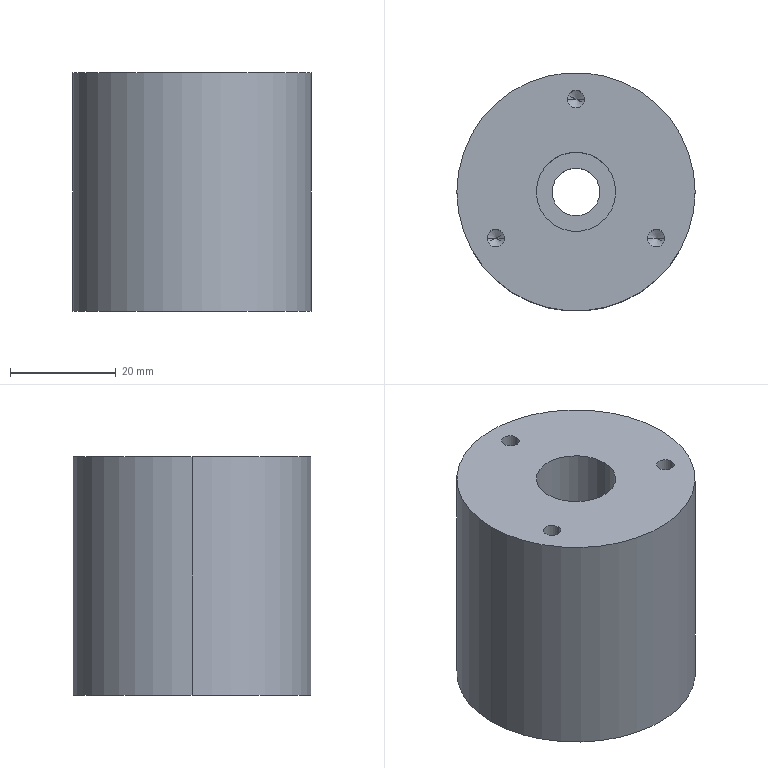Part | STEP file | Caster seat | 1 solid | 21 faces | box 45 x 45 x 45 mm | volume 66141 mm3 | cylinder 12 | cone 6 | plane 3 | commonest cylinder face diameters 3.3 x6 9 x2 15 x2 45 x2
STEP:
#1=CARTESIAN_POINT('',(0.,0.,0.));
#2=DIRECTION('',(0.,0.,1.));
#3=DIRECTION('',(1.,0.,0.));
#4=AXIS2_PLACEMENT_3D('',#1,#2,#3);
#5=CARTESIAN_POINT('',(7.5,0.,25.));
#6=VERTEX_POINT('',#5);
#7=CARTESIAN_POINT('',(7.5,0.,45.));
#8=VERTEX_POINT('',#7);
#9=CARTESIAN_POINT('',(7.5,0.,45.));
#10=DIRECTION('',(0.,0.,1.));
#11=VECTOR('',#10,1.);
#12=LINE('',#9,#11);
#13=CARTESIAN_POINT('',(0.,0.,45.));
#14=DIRECTION('',(0.,0.,1.));
#15=DIRECTION('',(1.,0.,0.));
#16=AXIS2_PLACEMENT_3D('',#13,#14,#15);
#17=CYLINDRICAL_SURFACE('',#16,7.5);
#18=CARTESIAN_POINT('',(6.283,0.));
#19=DIRECTION('',(0.,1.));
#20=VECTOR('',#19,1.);
#21=LINE('',#18,#20);
#22=(GEOMETRIC_REPRESENTATION_CONTEXT(2)PARAMETRIC_REPRESENTATION_CONTEXT()REPRESENTATION_CONTEXT('',''));
#23=DEFINITIONAL_REPRESENTATION('',(#21),#22);
#24=PCURVE('',#17,#23);
#25=CARTESIAN_POINT('',(0.,0.,45.));
#26=DIRECTION('',(0.,0.,1.));
#27=DIRECTION('',(1.,0.,0.));
#28=AXIS2_PLACEMENT_3D('',#25,#26,#27);
#29=CYLINDRICAL_SURFACE('',#28,7.5);
#30=CARTESIAN_POINT('',(0.,0.));
#31=DIRECTION('',(0.,1.));
#32=VECTOR('',#31,1.);
#33=LINE('',#30,#32);
#34=(GEOMETRIC_REPRESENTATION_CONTEXT(2)PARAMETRIC_REPRESENTATION_CONTEXT()REPRESENTATION_CONTEXT('',''));
#35=DEFINITIONAL_REPRESENTATION('',(#33),#34);
#36=PCURVE('',#29,#35);
#37=SURFACE_CURVE('',#12,(#24,#36),.PCURVE_S1.);
#38=EDGE_CURVE('',#6,#8,#37,.T.);
#39=ORIENTED_EDGE('',*,*,#38,.T.);
#40=CARTESIAN_POINT('',(-7.5,0.,45.));
#41=VERTEX_POINT('',#40);
#42=CARTESIAN_POINT('',(0.,0.,45.));
#43=DIRECTION('',(0.,0.,1.));
#44=DIRECTION('',(1.,0.,0.));
#45=AXIS2_PLACEMENT_3D('',#42,#43,#44);
#46=CIRCLE('',#45,7.5);
#47=CARTESIAN_POINT('',(0.,0.));
#48=DIRECTION('',(1.,0.));
#49=VECTOR('',#48,1.);
#50=LINE('',#47,#49);
#51=(GEOMETRIC_REPRESENTATION_CONTEXT(2)PARAMETRIC_REPRESENTATION_CONTEXT()REPRESENTATION_CONTEXT('',''));
#52=DEFINITIONAL_REPRESENTATION('',(#50),#51);
#53=PCURVE('',#17,#52);
#54=CARTESIAN_POINT('',(0.,0.,45.));
#55=DIRECTION('',(0.,0.,1.));
#56=DIRECTION('',(1.,0.,0.));
#57=AXIS2_PLACEMENT_3D('',#54,#55,#56);
#58=PLANE('',#57);
#59=CARTESIAN_POINT('',(0.,0.));
#60=DIRECTION('',(1.,0.));
#61=AXIS2_PLACEMENT_2D('',#59,#60);
#62=CIRCLE('',#61,7.5);
#63=(GEOMETRIC_REPRESENTATION_CONTEXT(2)PARAMETRIC_REPRESENTATION_CONTEXT()REPRESENTATION_CONTEXT('',''));
#64=DEFINITIONAL_REPRESENTATION('',(#62),#63);
#65=PCURVE('',#58,#64);
#66=SURFACE_CURVE('',#46,(#53,#65),.PCURVE_S1.);
#67=EDGE_CURVE('',#41,#8,#66,.T.);
#68=ORIENTED_EDGE('',*,*,#67,.F.);
#69=CARTESIAN_POINT('',(-7.5,0.,25.));
#70=VERTEX_POINT('',#69);
#71=CARTESIAN_POINT('',(-7.5,0.,45.));
#72=DIRECTION('',(0.,0.,1.));
#73=VECTOR('',#72,1.);
#74=LINE('',#71,#73);
#75=CARTESIAN_POINT('',(3.142,0.));
#76=DIRECTION('',(0.,1.));
#77=VECTOR('',#76,1.);
#78=LINE('',#75,#77);
#79=(GEOMETRIC_REPRESENTATION_CONTEXT(2)PARAMETRIC_REPRESENTATION_CONTEXT()REPRESENTATION_CONTEXT('',''));
#80=DEFINITIONAL_REPRESENTATION('',(#78),#79);
#81=PCURVE('',#17,#80);
#82=CARTESIAN_POINT('',(3.142,0.));
#83=DIRECTION('',(0.,1.));
#84=VECTOR('',#83,1.);
#85=LINE('',#82,#84);
#86=(GEOMETRIC_REPRESENTATION_CONTEXT(2)PARAMETRIC_REPRESENTATION_CONTEXT()REPRESENTATION_CONTEXT('',''));
#87=DEFINITIONAL_REPRESENTATION('',(#85),#86);
#88=PCURVE('',#29,#87);
#89=SURFACE_CURVE('',#74,(#81,#88),.PCURVE_S1.);
#90=EDGE_CURVE('',#70,#41,#89,.T.);
#91=ORIENTED_EDGE('',*,*,#90,.F.);
#92=CARTESIAN_POINT('',(0.,0.,25.));
#93=DIRECTION('',(0.,0.,1.));
#94=DIRECTION('',(1.,0.,0.));
#95=AXIS2_PLACEMENT_3D('',#92,#93,#94);
#96=CIRCLE('',#95,7.5);
#97=CARTESIAN_POINT('',(0.,-20.));
#98=DIRECTION('',(1.,0.));
#99=VECTOR('',#98,1.);
#100=LINE('',#97,#99);
#101=(GEOMETRIC_REPRESENTATION_CONTEXT(2)PARAMETRIC_REPRESENTATION_CONTEXT()REPRESENTATION_CONTEXT('',''));
#102=DEFINITIONAL_REPRESENTATION('',(#100),#101);
#103=PCURVE('',#17,#102);
#104=CARTESIAN_POINT('',(4.5,0.,25.));
#105=DIRECTION('',(0.,0.,-1.));
#106=DIRECTION('',(-1.,0.,0.));
#107=AXIS2_PLACEMENT_3D('',#104,#105,#106);
#108=PLANE('',#107);
#109=CARTESIAN_POINT('',(-3.,0.));
#110=CARTESIAN_POINT('',(-3.,12.99));
#111=CARTESIAN_POINT('',(8.25,6.495));
#112=CARTESIAN_POINT('',(19.5,0.));
#113=CARTESIAN_POINT('',(8.25,-6.495));
#114=CARTESIAN_POINT('',(-3.,-12.99));
#115=CARTESIAN_POINT('',(-3.,0.));
#116=(BOUNDED_CURVE()B_SPLINE_CURVE(2,(#109,#110,#111,#112,#113,#114,#115),.UNSPECIFIED.,.T.,.F.)B_SPLINE_CURVE_WITH_KNOTS((1,2,2,2,2,1),(-2.094,0.,2.094,4.189,6.283,8.378),.UNSPECIFIED.)CURVE()GEOMETRIC_REPRESENTATION_ITEM()RATIONAL_B_SPLINE_CURVE((1.,0.5,1.,0.5,1.,0.5,1.))REPRESENTATION_ITEM(''));
#117=(GEOMETRIC_REPRESENTATION_CONTEXT(2)PARAMETRIC_REPRESENTATION_CONTEXT()REPRESENTATION_CONTEXT('',''));
#118=DEFINITIONAL_REPRESENTATION('',(#116),#117);
#119=PCURVE('',#108,#118);
#120=SURFACE_CURVE('',#96,(#103,#119),.PCURVE_S1.);
#121=EDGE_CURVE('',#70,#6,#120,.T.);
#122=ORIENTED_EDGE('',*,*,#121,.T.);
#123=EDGE_LOOP('',(#39,#68,#91,#122));
#124=FACE_BOUND('',#123,.F.);
#125=ADVANCED_FACE('',(#124),#17,.F.);
#126=CARTESIAN_POINT('',(4.5,0.,0.));
#127=VERTEX_POINT('',#126);
#128=CARTESIAN_POINT('',(4.5,0.,25.));
#129=VERTEX_POINT('',#128);
#130=CARTESIAN_POINT('',(4.5,0.,45.));
#131=DIRECTION('',(0.,0.,1.));
#132=VECTOR('',#131,1.);
#133=LINE('',#130,#132);
#134=CARTESIAN_POINT('',(0.,0.,45.));
#135=DIRECTION('',(0.,0.,1.));
#136=DIRECTION('',(1.,0.,0.));
#137=AXIS2_PLACEMENT_3D('',#134,#135,#136);
#138=CYLINDRICAL_SURFACE('',#137,4.5);
#139=CARTESIAN_POINT('',(6.283,0.));
#140=DIRECTION('',(0.,1.));
#141=VECTOR('',#140,1.);
#142=LINE('',#139,#141);
#143=(GEOMETRIC_REPRESENTATION_CONTEXT(2)PARAMETRIC_REPRESENTATION_CONTEXT()REPRESENTATION_CONTEXT('',''));
#144=DEFINITIONAL_REPRESENTATION('',(#142),#143);
#145=PCURVE('',#138,#144);
#146=CARTESIAN_POINT('',(0.,0.,45.));
#147=DIRECTION('',(0.,0.,1.));
#148=DIRECTION('',(1.,0.,0.));
#149=AXIS2_PLACEMENT_3D('',#146,#147,#148);
#150=CYLINDRICAL_SURFACE('',#149,4.5);
#151=CARTESIAN_POINT('',(0.,0.));
#152=DIRECTION('',(0.,1.));
#153=VECTOR('',#152,1.);
#154=LINE('',#151,#153);
#155=(GEOMETRIC_REPRESENTATION_CONTEXT(2)PARAMETRIC_REPRESENTATION_CONTEXT()REPRESENTATION_CONTEXT('',''));
#156=DEFINITIONAL_REPRESENTATION('',(#154),#155);
#157=PCURVE('',#150,#156);
#158=SURFACE_CURVE('',#133,(#145,#157),.PCURVE_S1.);
#159=EDGE_CURVE('',#127,#129,#158,.T.);
#160=ORIENTED_EDGE('',*,*,#159,.T.);
#161=CARTESIAN_POINT('',(-4.5,0.,25.));
#162=VERTEX_POINT('',#161);
#163=CARTESIAN_POINT('',(0.,0.,25.));
#164=DIRECTION('',(0.,0.,1.));
#165=DIRECTION('',(1.,0.,0.));
#166=AXIS2_PLACEMENT_3D('',#163,#164,#165);
#167=CIRCLE('',#166,4.5);
#168=CARTESIAN_POINT('',(0.,-20.));
#169=DIRECTION('',(1.,0.));
#170=VECTOR('',#169,1.);
#171=LINE('',#168,#170);
#172=(GEOMETRIC_REPRESENTATION_CONTEXT(2)PARAMETRIC_REPRESENTATION_CONTEXT()REPRESENTATION_CONTEXT('',''));
#173=DEFINITIONAL_REPRESENTATION('',(#171),#172);
#174=PCURVE('',#138,#173);
#175=CARTESIAN_POINT('',(0.,0.));
#176=CARTESIAN_POINT('',(0.,7.794));
#177=CARTESIAN_POINT('',(6.75,3.897));
#178=CARTESIAN_POINT('',(13.5,0.));
#179=CARTESIAN_POINT('',(6.75,-3.897));
#180=CARTESIAN_POINT('',(0.,-7.794));
#181=CARTESIAN_POINT('',(0.,0.));
#182=(BOUNDED_CURVE()B_SPLINE_CURVE(2,(#175,#176,#177,#178,#179,#180,#181),.UNSPECIFIED.,.T.,.F.)B_SPLINE_CURVE_WITH_KNOTS((1,2,2,2,2,1),(-2.094,0.,2.094,4.189,6.283,8.378),.UNSPECIFIED.)CURVE()GEOMETRIC_REPRESENTATION_ITEM()RATIONAL_B_SPLINE_CURVE((1.,0.5,1.,0.5,1.,0.5,1.))REPRESENTATION_ITEM(''));
#183=(GEOMETRIC_REPRESENTATION_CONTEXT(2)PARAMETRIC_REPRESENTATION_CONTEXT()REPRESENTATION_CONTEXT('',''));
#184=DEFINITIONAL_REPRESENTATION('',(#182),#183);
#185=PCURVE('',#108,#184);
#186=SURFACE_CURVE('',#167,(#174,#185),.PCURVE_S1.);
#187=EDGE_CURVE('',#162,#129,#186,.T.);
#188=ORIENTED_EDGE('',*,*,#187,.F.);
#189=CARTESIAN_POINT('',(-4.5,0.,0.));
#190=VERTEX_POINT('',#189);
#191=CARTESIAN_POINT('',(-4.5,0.,45.));
#192=DIRECTION('',(0.,0.,1.));
#193=VECTOR('',#192,1.);
#194=LINE('',#191,#193);
#195=CARTESIAN_POINT('',(3.142,0.));
#196=DIRECTION('',(0.,1.));
#197=VECTOR('',#196,1.);
#198=LINE('',#195,#197);
#199=(GEOMETRIC_REPRESENTATION_CONTEXT(2)PARAMETRIC_REPRESENTATION_CONTEXT()REPRESENTATION_CONTEXT('',''));
#200=DEFINITIONAL_REPRESENTATION('',(#198),#199);
#201=PCURVE('',#138,#200);
#202=CARTESIAN_POINT('',(3.142,0.));
#203=DIRECTION('',(0.,1.));
#204=VECTOR('',#203,1.);
#205=LINE('',#202,#204);
#206=(GEOMETRIC_REPRESENTATION_CONTEXT(2)PARAMETRIC_REPRESENTATION_CONTEXT()REPRESENTATION_CONTEXT('',''));
#207=DEFINITIONAL_REPRESENTATION('',(#205),#206);
#208=PCURVE('',#150,#207);
#209=SURFACE_CURVE('',#194,(#201,#208),.PCURVE_S1.);
#210=EDGE_CURVE('',#190,#162,#209,.T.);
#211=ORIENTED_EDGE('',*,*,#210,.F.);
#212=CARTESIAN_POINT('',(0.,0.,0.));
#213=DIRECTION('',(0.,0.,1.));
#214=DIRECTION('',(1.,0.,0.));
#215=AXIS2_PLACEMENT_3D('',#212,#213,#214);
#216=CIRCLE('',#215,4.5);
#217=CARTESIAN_POINT('',(0.,-45.));
#218=DIRECTION('',(1.,0.));
#219=VECTOR('',#218,1.);
#220=LINE('',#217,#219);
#221=(GEOMETRIC_REPRESENTATION_CONTEXT(2)PARAMETRIC_REPRESENTATION_CONTEXT()REPRESENTATION_CONTEXT('',''));
#222=DEFINITIONAL_REPRESENTATION('',(#220),#221);
#223=PCURVE('',#138,#222);
#224=CARTESIAN_POINT('',(0.,0.,0.));
#225=DIRECTION('',(0.,0.,1.));
#226=DIRECTION('',(1.,0.,0.));
#227=AXIS2_PLACEMENT_3D('',#224,#225,#226);
#228=PLANE('',#227);
#229=CARTESIAN_POINT('',(0.,0.));
#230=DIRECTION('',(1.,0.));
#231=AXIS2_PLACEMENT_2D('',#229,#230);
#232=CIRCLE('',#231,4.5);
#233=(GEOMETRIC_REPRESENTATION_CONTEXT(2)PARAMETRIC_REPRESENTATION_CONTEXT()REPRESENTATION_CONTEXT('',''));
#234=DEFINITIONAL_REPRESENTATION('',(#232),#233);
#235=PCURVE('',#228,#234);
#236=SURFACE_CURVE('',#216,(#223,#235),.PCURVE_S1.);
#237=EDGE_CURVE('',#190,#127,#236,.T.);
#238=ORIENTED_EDGE('',*,*,#237,.T.);
#239=EDGE_LOOP('',(#160,#188,#211,#238));
#240=FACE_BOUND('',#239,.F.);
#241=ADVANCED_FACE('',(#240),#138,.F.);
#242=CARTESIAN_POINT('',(-13.505,-8.75,33.5));
#243=VERTEX_POINT('',#242);
#244=CARTESIAN_POINT('',(-13.505,-8.75,45.));
#245=VERTEX_POINT('',#244);
#246=CARTESIAN_POINT('',(-13.505,-8.75,45.));
#247=DIRECTION('',(0.,0.,1.));
#248=VECTOR('',#247,1.);
#249=LINE('',#246,#248);
#250=CARTESIAN_POINT('',(-15.155,-8.75,45.));
#251=DIRECTION('',(0.,0.,1.));
#252=DIRECTION('',(1.,0.,0.));
#253=AXIS2_PLACEMENT_3D('',#250,#251,#252);
#254=CYLINDRICAL_SURFACE('',#253,1.65);
#255=CARTESIAN_POINT('',(6.283,0.));
#256=DIRECTION('',(0.,1.));
#257=VECTOR('',#256,1.);
#258=LINE('',#255,#257);
#259=(GEOMETRIC_REPRESENTATION_CONTEXT(2)PARAMETRIC_REPRESENTATION_CONTEXT()REPRESENTATION_CONTEXT('',''));
#260=DEFINITIONAL_REPRESENTATION('',(#258),#259);
#261=PCURVE('',#254,#260);
#262=CARTESIAN_POINT('',(-15.155,-8.75,45.));
#263=DIRECTION('',(0.,0.,1.));
#264=DIRECTION('',(1.,0.,0.));
#265=AXIS2_PLACEMENT_3D('',#262,#263,#264);
#266=CYLINDRICAL_SURFACE('',#265,1.65);
#267=CARTESIAN_POINT('',(0.,0.));
#268=DIRECTION('',(0.,1.));
#269=VECTOR('',#268,1.);
#270=LINE('',#267,#269);
#271=(GEOMETRIC_REPRESENTATION_CONTEXT(2)PARAMETRIC_REPRESENTATION_CONTEXT()REPRESENTATION_CONTEXT('',''));
#272=DEFINITIONAL_REPRESENTATION('',(#270),#271);
#273=PCURVE('',#266,#272);
#274=SURFACE_CURVE('',#249,(#261,#273),.PCURVE_S1.);
#275=EDGE_CURVE('',#243,#245,#274,.T.);
#276=ORIENTED_EDGE('',*,*,#275,.T.);
#277=CARTESIAN_POINT('',(-16.805,-8.75,45.));
#278=VERTEX_POINT('',#277);
#279=CARTESIAN_POINT('',(-15.155,-8.75,45.));
#280=DIRECTION('',(0.,0.,1.));
#281=DIRECTION('',(1.,0.,0.));
#282=AXIS2_PLACEMENT_3D('',#279,#280,#281);
#283=CIRCLE('',#282,1.65);
#284=CARTESIAN_POINT('',(0.,0.));
#285=DIRECTION('',(1.,0.));
#286=VECTOR('',#285,1.);
#287=LINE('',#284,#286);
#288=(GEOMETRIC_REPRESENTATION_CONTEXT(2)PARAMETRIC_REPRESENTATION_CONTEXT()REPRESENTATION_CONTEXT('',''));
#289=DEFINITIONAL_REPRESENTATION('',(#287),#288);
#290=PCURVE('',#254,#289);
#291=CARTESIAN_POINT('',(-15.155,-8.75));
#292=DIRECTION('',(1.,0.));
#293=AXIS2_PLACEMENT_2D('',#291,#292);
#294=CIRCLE('',#293,1.65);
#295=(GEOMETRIC_REPRESENTATION_CONTEXT(2)PARAMETRIC_REPRESENTATION_CONTEXT()REPRESENTATION_CONTEXT('',''));
#296=DEFINITIONAL_REPRESENTATION('',(#294),#295);
#297=PCURVE('',#58,#296);
#298=SURFACE_CURVE('',#283,(#290,#297),.PCURVE_S1.);
#299=EDGE_CURVE('',#278,#245,#298,.T.);
#300=ORIENTED_EDGE('',*,*,#299,.F.);
#301=CARTESIAN_POINT('',(-16.805,-8.75,33.5));
#302=VERTEX_POINT('',#301);
#303=CARTESIAN_POINT('',(-16.805,-8.75,45.));
#304=DIRECTION('',(0.,0.,1.));
#305=VECTOR('',#304,1.);
#306=LINE('',#303,#305);
#307=CARTESIAN_POINT('',(3.142,0.));
#308=DIRECTION('',(0.,1.));
#309=VECTOR('',#308,1.);
#310=LINE('',#307,#309);
#311=(GEOMETRIC_REPRESENTATION_CONTEXT(2)PARAMETRIC_REPRESENTATION_CONTEXT()REPRESENTATION_CONTEXT('',''));
#312=DEFINITIONAL_REPRESENTATION('',(#310),#311);
#313=PCURVE('',#254,#312);
#314=CARTESIAN_POINT('',(3.142,0.));
#315=DIRECTION('',(0.,1.));
#316=VECTOR('',#315,1.);
#317=LINE('',#314,#316);
#318=(GEOMETRIC_REPRESENTATION_CONTEXT(2)PARAMETRIC_REPRESENTATION_CONTEXT()REPRESENTATION_CONTEXT('',''));
#319=DEFINITIONAL_REPRESENTATION('',(#317),#318);
#320=PCURVE('',#266,#319);
#321=SURFACE_CURVE('',#306,(#313,#320),.PCURVE_S1.);
#322=EDGE_CURVE('',#302,#278,#321,.T.);
#323=ORIENTED_EDGE('',*,*,#322,.F.);
#324=CARTESIAN_POINT('',(-15.155,-8.75,33.5));
#325=DIRECTION('',(0.,0.,1.));
#326=DIRECTION('',(1.,0.,0.));
#327=AXIS2_PLACEMENT_3D('',#324,#325,#326);
#328=CIRCLE('',#327,1.65);
#329=CARTESIAN_POINT('',(0.,-11.5));
#330=DIRECTION('',(1.,0.));
#331=VECTOR('',#330,1.);
#332=LINE('',#329,#331);
#333=(GEOMETRIC_REPRESENTATION_CONTEXT(2)PARAMETRIC_REPRESENTATION_CONTEXT()REPRESENTATION_CONTEXT('',''));
#334=DEFINITIONAL_REPRESENTATION('',(#332),#333);
#335=PCURVE('',#254,#334);
#336=CARTESIAN_POINT('',(-15.155,-8.75,33.5));
#337=DIRECTION('',(0.,0.,1.));
#338=DIRECTION('',(1.,0.,0.));
#339=AXIS2_PLACEMENT_3D('',#336,#337,#338);
#340=CONICAL_SURFACE('',#339,1.65,1.03);
#341=CARTESIAN_POINT('',(0.,0.));
#342=DIRECTION('',(1.,0.));
#343=VECTOR('',#342,1.);
#344=LINE('',#341,#343);
#345=(GEOMETRIC_REPRESENTATION_CONTEXT(2)PARAMETRIC_REPRESENTATION_CONTEXT()REPRESENTATION_CONTEXT('',''));
#346=DEFINITIONAL_REPRESENTATION('',(#344),#345);
#347=PCURVE('',#340,#346);
#348=SURFACE_CURVE('',#328,(#335,#347),.PCURVE_S1.);
#349=EDGE_CURVE('',#302,#243,#348,.T.);
#350=ORIENTED_EDGE('',*,*,#349,.T.);
#351=EDGE_LOOP('',(#276,#300,#323,#350));
#352=FACE_BOUND('',#351,.F.);
#353=ADVANCED_FACE('',(#352),#254,.F.);
#354=ORIENTED_EDGE('',*,*,#349,.F.);
#355=CARTESIAN_POINT('',(-15.155,-8.75,32.509));
#356=VERTEX_POINT('',#355);
#357=CARTESIAN_POINT('',(-16.805,-8.75,33.5));
#358=DIRECTION('',(-0.8572,0.,0.515));
#359=VECTOR('',#358,1.);
#360=LINE('',#357,#359);
#361=CARTESIAN_POINT('',(3.142,0.));
#362=DIRECTION('',(0.,1.));
#363=VECTOR('',#362,1.);
#364=LINE('',#361,#363);
#365=(GEOMETRIC_REPRESENTATION_CONTEXT(2)PARAMETRIC_REPRESENTATION_CONTEXT()REPRESENTATION_CONTEXT('',''));
#366=DEFINITIONAL_REPRESENTATION('',(#364),#365);
#367=PCURVE('',#340,#366);
#368=CARTESIAN_POINT('',(-15.155,-8.75,33.5));
#369=DIRECTION('',(0.,0.,1.));
#370=DIRECTION('',(1.,0.,0.));
#371=AXIS2_PLACEMENT_3D('',#368,#369,#370);
#372=CONICAL_SURFACE('',#371,1.65,1.03);
#373=CARTESIAN_POINT('',(3.142,0.));
#374=DIRECTION('',(0.,1.));
#375=VECTOR('',#374,1.);
#376=LINE('',#373,#375);
#377=(GEOMETRIC_REPRESENTATION_CONTEXT(2)PARAMETRIC_REPRESENTATION_CONTEXT()REPRESENTATION_CONTEXT('',''));
#378=DEFINITIONAL_REPRESENTATION('',(#376),#377);
#379=PCURVE('',#372,#378);
#380=SURFACE_CURVE('',#360,(#367,#379),.PCURVE_S1.);
#381=EDGE_CURVE('',#356,#302,#380,.T.);
#382=ORIENTED_EDGE('',*,*,#381,.F.);
#383=CARTESIAN_POINT('',(-13.505,-8.75,33.5));
#384=DIRECTION('',(0.8572,0.,0.515));
#385=VECTOR('',#384,1.);
#386=LINE('',#383,#385);
#387=CARTESIAN_POINT('',(6.283,0.));
#388=DIRECTION('',(0.,1.));
#389=VECTOR('',#388,1.);
#390=LINE('',#387,#389);
#391=(GEOMETRIC_REPRESENTATION_CONTEXT(2)PARAMETRIC_REPRESENTATION_CONTEXT()REPRESENTATION_CONTEXT('',''));
#392=DEFINITIONAL_REPRESENTATION('',(#390),#391);
#393=PCURVE('',#340,#392);
#394=CARTESIAN_POINT('',(0.,0.));
#395=DIRECTION('',(0.,1.));
#396=VECTOR('',#395,1.);
#397=LINE('',#394,#396);
#398=(GEOMETRIC_REPRESENTATION_CONTEXT(2)PARAMETRIC_REPRESENTATION_CONTEXT()REPRESENTATION_CONTEXT('',''));
#399=DEFINITIONAL_REPRESENTATION('',(#397),#398);
#400=PCURVE('',#372,#399);
#401=SURFACE_CURVE('',#386,(#393,#400),.PCURVE_S1.);
#402=EDGE_CURVE('',#356,#243,#401,.T.);
#403=ORIENTED_EDGE('',*,*,#402,.T.);
#404=EDGE_LOOP('',(#354,#382,#403));
#405=FACE_BOUND('',#404,.F.);
#406=ADVANCED_FACE('',(#405),#340,.F.);
#407=CARTESIAN_POINT('',(16.805,-8.75,33.5));
#408=VERTEX_POINT('',#407);
#409=CARTESIAN_POINT('',(16.805,-8.75,45.));
#410=VERTEX_POINT('',#409);
#411=CARTESIAN_POINT('',(16.805,-8.75,45.));
#412=DIRECTION('',(0.,0.,1.));
#413=VECTOR('',#412,1.);
#414=LINE('',#411,#413);
#415=CARTESIAN_POINT('',(15.155,-8.75,45.));
#416=DIRECTION('',(0.,0.,1.));
#417=DIRECTION('',(1.,0.,0.));
#418=AXIS2_PLACEMENT_3D('',#415,#416,#417);
#419=CYLINDRICAL_SURFACE('',#418,1.65);
#420=CARTESIAN_POINT('',(6.283,0.));
#421=DIRECTION('',(0.,1.));
#422=VECTOR('',#421,1.);
#423=LINE('',#420,#422);
#424=(GEOMETRIC_REPRESENTATION_CONTEXT(2)PARAMETRIC_REPRESENTATION_CONTEXT()REPRESENTATION_CONTEXT('',''));
#425=DEFINITIONAL_REPRESENTATION('',(#423),#424);
#426=PCURVE('',#419,#425);
#427=CARTESIAN_POINT('',(15.155,-8.75,45.));
#428=DIRECTION('',(0.,0.,1.));
#429=DIRECTION('',(1.,0.,0.));
#430=AXIS2_PLACEMENT_3D('',#427,#428,#429);
#431=CYLINDRICAL_SURFACE('',#430,1.65);
#432=CARTESIAN_POINT('',(0.,0.));
#433=DIRECTION('',(0.,1.));
#434=VECTOR('',#433,1.);
#435=LINE('',#432,#434);
#436=(GEOMETRIC_REPRESENTATION_CONTEXT(2)PARAMETRIC_REPRESENTATION_CONTEXT()REPRESENTATION_CONTEXT('',''));
#437=DEFINITIONAL_REPRESENTATION('',(#435),#436);
#438=PCURVE('',#431,#437);
#439=SURFACE_CURVE('',#414,(#426,#438),.PCURVE_S1.);
#440=EDGE_CURVE('',#408,#410,#439,.T.);
#441=ORIENTED_EDGE('',*,*,#440,.T.);
#442=CARTESIAN_POINT('',(13.505,-8.75,45.));
#443=VERTEX_POINT('',#442);
#444=CARTESIAN_POINT('',(15.155,-8.75,45.));
#445=DIRECTION('',(0.,0.,1.));
#446=DIRECTION('',(1.,0.,0.));
#447=AXIS2_PLACEMENT_3D('',#444,#445,#446);
#448=CIRCLE('',#447,1.65);
#449=CARTESIAN_POINT('',(0.,0.));
#450=DIRECTION('',(1.,0.));
#451=VECTOR('',#450,1.);
#452=LINE('',#449,#451);
#453=(GEOMETRIC_REPRESENTATION_CONTEXT(2)PARAMETRIC_REPRESENTATION_CONTEXT()REPRESENTATION_CONTEXT('',''));
#454=DEFINITIONAL_REPRESENTATION('',(#452),#453);
#455=PCURVE('',#419,#454);
#456=CARTESIAN_POINT('',(15.155,-8.75));
#457=DIRECTION('',(1.,0.));
#458=AXIS2_PLACEMENT_2D('',#456,#457);
#459=CIRCLE('',#458,1.65);
#460=(GEOMETRIC_REPRESENTATION_CONTEXT(2)PARAMETRIC_REPRESENTATION_CONTEXT()REPRESENTATION_CONTEXT('',''));
#461=DEFINITIONAL_REPRESENTATION('',(#459),#460);
#462=PCURVE('',#58,#461);
#463=SURFACE_CURVE('',#448,(#455,#462),.PCURVE_S1.);
#464=EDGE_CURVE('',#443,#410,#463,.T.);
#465=ORIENTED_EDGE('',*,*,#464,.F.);
#466=CARTESIAN_POINT('',(13.505,-8.75,33.5));
#467=VERTEX_POINT('',#466);
#468=CARTESIAN_POINT('',(13.505,-8.75,45.));
#469=DIRECTION('',(0.,0.,1.));
#470=VECTOR('',#469,1.);
#471=LINE('',#468,#470);
#472=CARTESIAN_POINT('',(3.142,0.));
#473=DIRECTION('',(0.,1.));
#474=VECTOR('',#473,1.);
#475=LINE('',#472,#474);
#476=(GEOMETRIC_REPRESENTATION_CONTEXT(2)PARAMETRIC_REPRESENTATION_CONTEXT()REPRESENTATION_CONTEXT('',''));
#477=DEFINITIONAL_REPRESENTATION('',(#475),#476);
#478=PCURVE('',#419,#477);
#479=CARTESIAN_POINT('',(3.142,0.));
#480=DIRECTION('',(0.,1.));
#481=VECTOR('',#480,1.);
#482=LINE('',#479,#481);
#483=(GEOMETRIC_REPRESENTATION_CONTEXT(2)PARAMETRIC_REPRESENTATION_CONTEXT()REPRESENTATION_CONTEXT('',''));
#484=DEFINITIONAL_REPRESENTATION('',(#482),#483);
#485=PCURVE('',#431,#484);
#486=SURFACE_CURVE('',#471,(#478,#485),.PCURVE_S1.);
#487=EDGE_CURVE('',#467,#443,#486,.T.);
#488=ORIENTED_EDGE('',*,*,#487,.F.);
#489=CARTESIAN_POINT('',(15.155,-8.75,33.5));
#490=DIRECTION('',(0.,0.,1.));
#491=DIRECTION('',(1.,0.,0.));
#492=AXIS2_PLACEMENT_3D('',#489,#490,#491);
#493=CIRCLE('',#492,1.65);
#494=CARTESIAN_POINT('',(0.,-11.5));
#495=DIRECTION('',(1.,0.));
#496=VECTOR('',#495,1.);
#497=LINE('',#494,#496);
#498=(GEOMETRIC_REPRESENTATION_CONTEXT(2)PARAMETRIC_REPRESENTATION_CONTEXT()REPRESENTATION_CONTEXT('',''));
#499=DEFINITIONAL_REPRESENTATION('',(#497),#498);
#500=PCURVE('',#419,#499);
#501=CARTESIAN_POINT('',(15.155,-8.75,33.5));
#502=DIRECTION('',(0.,0.,1.));
#503=DIRECTION('',(1.,0.,0.));
#504=AXIS2_PLACEMENT_3D('',#501,#502,#503);
#505=CONICAL_SURFACE('',#504,1.65,1.03);
#506=CARTESIAN_POINT('',(0.,0.));
#507=DIRECTION('',(1.,0.));
#508=VECTOR('',#507,1.);
#509=LINE('',#506,#508);
#510=(GEOMETRIC_REPRESENTATION_CONTEXT(2)PARAMETRIC_REPRESENTATION_CONTEXT()REPRESENTATION_CONTEXT('',''));
#511=DEFINITIONAL_REPRESENTATION('',(#509),#510);
#512=PCURVE('',#505,#511);
#513=SURFACE_CURVE('',#493,(#500,#512),.PCURVE_S1.);
#514=EDGE_CURVE('',#467,#408,#513,.T.);
#515=ORIENTED_EDGE('',*,*,#514,.T.);
#516=EDGE_LOOP('',(#441,#465,#488,#515));
#517=FACE_BOUND('',#516,.F.);
#518=ADVANCED_FACE('',(#517),#419,.F.);
#519=ORIENTED_EDGE('',*,*,#514,.F.);
#520=CARTESIAN_POINT('',(15.155,-8.75,32.509));
#521=VERTEX_POINT('',#520);
#522=CARTESIAN_POINT('',(13.505,-8.75,33.5));
#523=DIRECTION('',(-0.8572,0.,0.515));
#524=VECTOR('',#523,1.);
#525=LINE('',#522,#524);
#526=CARTESIAN_POINT('',(3.142,0.));
#527=DIRECTION('',(0.,1.));
#528=VECTOR('',#527,1.);
#529=LINE('',#526,#528);
#530=(GEOMETRIC_REPRESENTATION_CONTEXT(2)PARAMETRIC_REPRESENTATION_CONTEXT()REPRESENTATION_CONTEXT('',''));
#531=DEFINITIONAL_REPRESENTATION('',(#529),#530);
#532=PCURVE('',#505,#531);
#533=CARTESIAN_POINT('',(15.155,-8.75,33.5));
#534=DIRECTION('',(0.,0.,1.));
#535=DIRECTION('',(1.,0.,0.));
#536=AXIS2_PLACEMENT_3D('',#533,#534,#535);
#537=CONICAL_SURFACE('',#536,1.65,1.03);
#538=CARTESIAN_POINT('',(3.142,0.));
#539=DIRECTION('',(0.,1.));
#540=VECTOR('',#539,1.);
#541=LINE('',#538,#540);
#542=(GEOMETRIC_REPRESENTATION_CONTEXT(2)PARAMETRIC_REPRESENTATION_CONTEXT()REPRESENTATION_CONTEXT('',''));
#543=DEFINITIONAL_REPRESENTATION('',(#541),#542);
#544=PCURVE('',#537,#543);
#545=SURFACE_CURVE('',#525,(#532,#544),.PCURVE_S1.);
#546=EDGE_CURVE('',#521,#467,#545,.T.);
#547=ORIENTED_EDGE('',*,*,#546,.F.);
#548=CARTESIAN_POINT('',(16.805,-8.75,33.5));
#549=DIRECTION('',(0.8572,0.,0.515));
#550=VECTOR('',#549,1.);
#551=LINE('',#548,#550);
#552=CARTESIAN_POINT('',(6.283,0.));
#553=DIRECTION('',(0.,1.));
#554=VECTOR('',#553,1.);
#555=LINE('',#552,#554);
#556=(GEOMETRIC_REPRESENTATION_CONTEXT(2)PARAMETRIC_REPRESENTATION_CONTEXT()REPRESENTATION_CONTEXT('',''));
#557=DEFINITIONAL_REPRESENTATION('',(#555),#556);
#558=PCURVE('',#505,#557);
#559=CARTESIAN_POINT('',(0.,0.));
#560=DIRECTION('',(0.,1.));
#561=VECTOR('',#560,1.);
#562=LINE('',#559,#561);
#563=(GEOMETRIC_REPRESENTATION_CONTEXT(2)PARAMETRIC_REPRESENTATION_CONTEXT()REPRESENTATION_CONTEXT('',''));
#564=DEFINITIONAL_REPRESENTATION('',(#562),#563);
#565=PCURVE('',#537,#564);
#566=SURFACE_CURVE('',#551,(#558,#565),.PCURVE_S1.);
#567=EDGE_CURVE('',#521,#408,#566,.T.);
#568=ORIENTED_EDGE('',*,*,#567,.T.);
#569=EDGE_LOOP('',(#519,#547,#568));
#570=FACE_BOUND('',#569,.F.);
#571=ADVANCED_FACE('',(#570),#505,.F.);
#572=CARTESIAN_POINT('',(1.65,17.5,33.5));
#573=VERTEX_POINT('',#572);
#574=CARTESIAN_POINT('',(1.65,17.5,45.));
#575=VERTEX_POINT('',#574);
#576=CARTESIAN_POINT('',(1.65,17.5,45.));
#577=DIRECTION('',(0.,0.,1.));
#578=VECTOR('',#577,1.);
#579=LINE('',#576,#578);
#580=CARTESIAN_POINT('',(0.,17.5,45.));
#581=DIRECTION('',(0.,0.,1.));
#582=DIRECTION('',(1.,0.,0.));
#583=AXIS2_PLACEMENT_3D('',#580,#581,#582);
#584=CYLINDRICAL_SURFACE('',#583,1.65);
#585=CARTESIAN_POINT('',(6.283,0.));
#586=DIRECTION('',(0.,1.));
#587=VECTOR('',#586,1.);
#588=LINE('',#585,#587);
#589=(GEOMETRIC_REPRESENTATION_CONTEXT(2)PARAMETRIC_REPRESENTATION_CONTEXT()REPRESENTATION_CONTEXT('',''));
#590=DEFINITIONAL_REPRESENTATION('',(#588),#589);
#591=PCURVE('',#584,#590);
#592=CARTESIAN_POINT('',(0.,17.5,45.));
#593=DIRECTION('',(0.,0.,1.));
#594=DIRECTION('',(1.,0.,0.));
#595=AXIS2_PLACEMENT_3D('',#592,#593,#594);
#596=CYLINDRICAL_SURFACE('',#595,1.65);
#597=CARTESIAN_POINT('',(0.,0.));
#598=DIRECTION('',(0.,1.));
#599=VECTOR('',#598,1.);
#600=LINE('',#597,#599);
#601=(GEOMETRIC_REPRESENTATION_CONTEXT(2)PARAMETRIC_REPRESENTATION_CONTEXT()REPRESENTATION_CONTEXT('',''));
#602=DEFINITIONAL_REPRESENTATION('',(#600),#601);
#603=PCURVE('',#596,#602);
#604=SURFACE_CURVE('',#579,(#591,#603),.PCURVE_S1.);
#605=EDGE_CURVE('',#573,#575,#604,.T.);
#606=ORIENTED_EDGE('',*,*,#605,.T.);
#607=CARTESIAN_POINT('',(-1.65,17.5,45.));
#608=VERTEX_POINT('',#607);
#609=CARTESIAN_POINT('',(0.,17.5,45.));
#610=DIRECTION('',(0.,0.,1.));
#611=DIRECTION('',(1.,0.,0.));
#612=AXIS2_PLACEMENT_3D('',#609,#610,#611);
#613=CIRCLE('',#612,1.65);
#614=CARTESIAN_POINT('',(0.,0.));
#615=DIRECTION('',(1.,0.));
#616=VECTOR('',#615,1.);
#617=LINE('',#614,#616);
#618=(GEOMETRIC_REPRESENTATION_CONTEXT(2)PARAMETRIC_REPRESENTATION_CONTEXT()REPRESENTATION_CONTEXT('',''));
#619=DEFINITIONAL_REPRESENTATION('',(#617),#618);
#620=PCURVE('',#584,#619);
#621=CARTESIAN_POINT('',(0.,17.5));
#622=DIRECTION('',(1.,0.));
#623=AXIS2_PLACEMENT_2D('',#621,#622);
#624=CIRCLE('',#623,1.65);
#625=(GEOMETRIC_REPRESENTATION_CONTEXT(2)PARAMETRIC_REPRESENTATION_CONTEXT()REPRESENTATION_CONTEXT('',''));
#626=DEFINITIONAL_REPRESENTATION('',(#624),#625);
#627=PCURVE('',#58,#626);
#628=SURFACE_CURVE('',#613,(#620,#627),.PCURVE_S1.);
#629=EDGE_CURVE('',#608,#575,#628,.T.);
#630=ORIENTED_EDGE('',*,*,#629,.F.);
#631=CARTESIAN_POINT('',(-1.65,17.5,33.5));
#632=VERTEX_POINT('',#631);
#633=CARTESIAN_POINT('',(-1.65,17.5,45.));
#634=DIRECTION('',(0.,0.,1.));
#635=VECTOR('',#634,1.);
#636=LINE('',#633,#635);
#637=CARTESIAN_POINT('',(3.142,0.));
#638=DIRECTION('',(0.,1.));
#639=VECTOR('',#638,1.);
#640=LINE('',#637,#639);
#641=(GEOMETRIC_REPRESENTATION_CONTEXT(2)PARAMETRIC_REPRESENTATION_CONTEXT()REPRESENTATION_CONTEXT('',''));
#642=DEFINITIONAL_REPRESENTATION('',(#640),#641);
#643=PCURVE('',#584,#642);
#644=CARTESIAN_POINT('',(3.142,0.));
#645=DIRECTION('',(0.,1.));
#646=VECTOR('',#645,1.);
#647=LINE('',#644,#646);
#648=(GEOMETRIC_REPRESENTATION_CONTEXT(2)PARAMETRIC_REPRESENTATION_CONTEXT()REPRESENTATION_CONTEXT('',''));
#649=DEFINITIONAL_REPRESENTATION('',(#647),#648);
#650=PCURVE('',#596,#649);
#651=SURFACE_CURVE('',#636,(#643,#650),.PCURVE_S1.);
#652=EDGE_CURVE('',#632,#608,#651,.T.);
#653=ORIENTED_EDGE('',*,*,#652,.F.);
#654=CARTESIAN_POINT('',(0.,17.5,33.5));
#655=DIRECTION('',(0.,0.,1.));
#656=DIRECTION('',(1.,0.,0.));
#657=AXIS2_PLACEMENT_3D('',#654,#655,#656);
#658=CIRCLE('',#657,1.65);
#659=CARTESIAN_POINT('',(0.,-11.5));
#660=DIRECTION('',(1.,0.));
#661=VECTOR('',#660,1.);
#662=LINE('',#659,#661);
#663=(GEOMETRIC_REPRESENTATION_CONTEXT(2)PARAMETRIC_REPRESENTATION_CONTEXT()REPRESENTATION_CONTEXT('',''));
#664=DEFINITIONAL_REPRESENTATION('',(#662),#663);
#665=PCURVE('',#584,#664);
#666=CARTESIAN_POINT('',(0.,17.5,33.5));
#667=DIRECTION('',(0.,0.,1.));
#668=DIRECTION('',(1.,0.,0.));
#669=AXIS2_PLACEMENT_3D('',#666,#667,#668);
#670=CONICAL_SURFACE('',#669,1.65,1.03);
#671=CARTESIAN_POINT('',(0.,0.));
#672=DIRECTION('',(1.,0.));
#673=VECTOR('',#672,1.);
#674=LINE('',#671,#673);
#675=(GEOMETRIC_REPRESENTATION_CONTEXT(2)PARAMETRIC_REPRESENTATION_CONTEXT()REPRESENTATION_CONTEXT('',''));
#676=DEFINITIONAL_REPRESENTATION('',(#674),#675);
#677=PCURVE('',#670,#676);
#678=SURFACE_CURVE('',#658,(#665,#677),.PCURVE_S1.);
#679=EDGE_CURVE('',#632,#573,#678,.T.);
#680=ORIENTED_EDGE('',*,*,#679,.T.);
#681=EDGE_LOOP('',(#606,#630,#653,#680));
#682=FACE_BOUND('',#681,.F.);
#683=ADVANCED_FACE('',(#682),#584,.F.);
#684=ORIENTED_EDGE('',*,*,#679,.F.);
#685=CARTESIAN_POINT('',(0.,17.5,32.509));
#686=VERTEX_POINT('',#685);
#687=CARTESIAN_POINT('',(-1.65,17.5,33.5));
#688=DIRECTION('',(-0.8572,0.,0.515));
#689=VECTOR('',#688,1.);
#690=LINE('',#687,#689);
#691=CARTESIAN_POINT('',(3.142,0.));
#692=DIRECTION('',(0.,1.));
#693=VECTOR('',#692,1.);
#694=LINE('',#691,#693);
#695=(GEOMETRIC_REPRESENTATION_CONTEXT(2)PARAMETRIC_REPRESENTATION_CONTEXT()REPRESENTATION_CONTEXT('',''));
#696=DEFINITIONAL_REPRESENTATION('',(#694),#695);
#697=PCURVE('',#670,#696);
#698=CARTESIAN_POINT('',(0.,17.5,33.5));
#699=DIRECTION('',(0.,0.,1.));
#700=DIRECTION('',(1.,0.,0.));
#701=AXIS2_PLACEMENT_3D('',#698,#699,#700);
#702=CONICAL_SURFACE('',#701,1.65,1.03);
#703=CARTESIAN_POINT('',(3.142,0.));
#704=DIRECTION('',(0.,1.));
#705=VECTOR('',#704,1.);
#706=LINE('',#703,#705);
#707=(GEOMETRIC_REPRESENTATION_CONTEXT(2)PARAMETRIC_REPRESENTATION_CONTEXT()REPRESENTATION_CONTEXT('',''));
#708=DEFINITIONAL_REPRESENTATION('',(#706),#707);
#709=PCURVE('',#702,#708);
#710=SURFACE_CURVE('',#690,(#697,#709),.PCURVE_S1.);
#711=EDGE_CURVE('',#686,#632,#710,.T.);
#712=ORIENTED_EDGE('',*,*,#711,.F.);
#713=CARTESIAN_POINT('',(1.65,17.5,33.5));
#714=DIRECTION('',(0.8572,0.,0.515));
#715=VECTOR('',#714,1.);
#716=LINE('',#713,#715);
#717=CARTESIAN_POINT('',(6.283,0.));
#718=DIRECTION('',(0.,1.));
#719=VECTOR('',#718,1.);
#720=LINE('',#717,#719);
#721=(GEOMETRIC_REPRESENTATION_CONTEXT(2)PARAMETRIC_REPRESENTATION_CONTEXT()REPRESENTATION_CONTEXT('',''));
#722=DEFINITIONAL_REPRESENTATION('',(#720),#721);
#723=PCURVE('',#670,#722);
#724=CARTESIAN_POINT('',(0.,0.));
#725=DIRECTION('',(0.,1.));
#726=VECTOR('',#725,1.);
#727=LINE('',#724,#726);
#728=(GEOMETRIC_REPRESENTATION_CONTEXT(2)PARAMETRIC_REPRESENTATION_CONTEXT()REPRESENTATION_CONTEXT('',''));
#729=DEFINITIONAL_REPRESENTATION('',(#727),#728);
#730=PCURVE('',#702,#729);
#731=SURFACE_CURVE('',#716,(#723,#730),.PCURVE_S1.);
#732=EDGE_CURVE('',#686,#573,#731,.T.);
#733=ORIENTED_EDGE('',*,*,#732,.T.);
#734=EDGE_LOOP('',(#684,#712,#733));
#735=FACE_BOUND('',#734,.F.);
#736=ADVANCED_FACE('',(#735),#670,.F.);
#737=CARTESIAN_POINT('',(22.5,0.,45.));
#738=VERTEX_POINT('',#737);
#739=CARTESIAN_POINT('',(-22.5,0.,45.));
#740=VERTEX_POINT('',#739);
#741=CARTESIAN_POINT('',(0.,0.,45.));
#742=DIRECTION('',(0.,0.,1.));
#743=DIRECTION('',(1.,0.,0.));
#744=AXIS2_PLACEMENT_3D('',#741,#742,#743);
#745=CIRCLE('',#744,22.5);
#746=CARTESIAN_POINT('',(0.,0.,45.));
#747=DIRECTION('',(0.,0.,-1.));
#748=DIRECTION('',(-1.,0.,0.));
#749=AXIS2_PLACEMENT_3D('',#746,#747,#748);
#750=CYLINDRICAL_SURFACE('',#749,22.5);
#751=CARTESIAN_POINT('',(3.142,0.));
#752=DIRECTION('',(-1.,0.));
#753=VECTOR('',#752,1.);
#754=LINE('',#751,#753);
#755=(GEOMETRIC_REPRESENTATION_CONTEXT(2)PARAMETRIC_REPRESENTATION_CONTEXT()REPRESENTATION_CONTEXT('',''));
#756=DEFINITIONAL_REPRESENTATION('',(#754),#755);
#757=PCURVE('',#750,#756);
#758=CARTESIAN_POINT('',(0.,0.));
#759=DIRECTION('',(1.,0.));
#760=AXIS2_PLACEMENT_2D('',#758,#759);
#761=CIRCLE('',#760,22.5);
#762=(GEOMETRIC_REPRESENTATION_CONTEXT(2)PARAMETRIC_REPRESENTATION_CONTEXT()REPRESENTATION_CONTEXT('',''));
#763=DEFINITIONAL_REPRESENTATION('',(#761),#762);
#764=PCURVE('',#58,#763);
#765=SURFACE_CURVE('',#745,(#757,#764),.PCURVE_S1.);
#766=EDGE_CURVE('',#738,#740,#765,.T.);
#767=ORIENTED_EDGE('',*,*,#766,.F.);
#768=CARTESIAN_POINT('',(22.5,0.,0.));
#769=VERTEX_POINT('',#768);
#770=CARTESIAN_POINT('',(22.5,0.,45.));
#771=DIRECTION('',(0.,0.,-1.));
#772=VECTOR('',#771,1.);
#773=LINE('',#770,#772);
#774=CARTESIAN_POINT('',(3.142,0.));
#775=DIRECTION('',(0.,1.));
#776=VECTOR('',#775,1.);
#777=LINE('',#774,#776);
#778=(GEOMETRIC_REPRESENTATION_CONTEXT(2)PARAMETRIC_REPRESENTATION_CONTEXT()REPRESENTATION_CONTEXT('',''));
#779=DEFINITIONAL_REPRESENTATION('',(#777),#778);
#780=PCURVE('',#750,#779);
#781=CARTESIAN_POINT('',(0.,0.,45.));
#782=DIRECTION('',(0.,0.,-1.));
#783=DIRECTION('',(-1.,0.,0.));
#784=AXIS2_PLACEMENT_3D('',#781,#782,#783);
#785=CYLINDRICAL_SURFACE('',#784,22.5);
#786=CARTESIAN_POINT('',(3.142,0.));
#787=DIRECTION('',(0.,1.));
#788=VECTOR('',#787,1.);
#789=LINE('',#786,#788);
#790=(GEOMETRIC_REPRESENTATION_CONTEXT(2)PARAMETRIC_REPRESENTATION_CONTEXT()REPRESENTATION_CONTEXT('',''));
#791=DEFINITIONAL_REPRESENTATION('',(#789),#790);
#792=PCURVE('',#785,#791);
#793=SURFACE_CURVE('',#773,(#780,#792),.PCURVE_S1.);
#794=EDGE_CURVE('',#738,#769,#793,.T.);
#795=ORIENTED_EDGE('',*,*,#794,.T.);
#796=CARTESIAN_POINT('',(-22.5,0.,0.));
#797=VERTEX_POINT('',#796);
#798=CARTESIAN_POINT('',(0.,0.,0.));
#799=DIRECTION('',(0.,0.,1.));
#800=DIRECTION('',(1.,0.,0.));
#801=AXIS2_PLACEMENT_3D('',#798,#799,#800);
#802=CIRCLE('',#801,22.5);
#803=CARTESIAN_POINT('',(3.142,45.));
#804=DIRECTION('',(-1.,0.));
#805=VECTOR('',#804,1.);
#806=LINE('',#803,#805);
#807=(GEOMETRIC_REPRESENTATION_CONTEXT(2)PARAMETRIC_REPRESENTATION_CONTEXT()REPRESENTATION_CONTEXT('',''));
#808=DEFINITIONAL_REPRESENTATION('',(#806),#807);
#809=PCURVE('',#750,#808);
#810=CARTESIAN_POINT('',(0.,0.));
#811=DIRECTION('',(1.,0.));
#812=AXIS2_PLACEMENT_2D('',#810,#811);
#813=CIRCLE('',#812,22.5);
#814=(GEOMETRIC_REPRESENTATION_CONTEXT(2)PARAMETRIC_REPRESENTATION_CONTEXT()REPRESENTATION_CONTEXT('',''));
#815=DEFINITIONAL_REPRESENTATION('',(#813),#814);
#816=PCURVE('',#228,#815);
#817=SURFACE_CURVE('',#802,(#809,#816),.PCURVE_S1.);
#818=EDGE_CURVE('',#769,#797,#817,.T.);
#819=ORIENTED_EDGE('',*,*,#818,.T.);
#820=CARTESIAN_POINT('',(-22.5,0.,45.));
#821=DIRECTION('',(0.,0.,-1.));
#822=VECTOR('',#821,1.);
#823=LINE('',#820,#822);
#824=CARTESIAN_POINT('',(0.,0.));
#825=DIRECTION('',(0.,1.));
#826=VECTOR('',#825,1.);
#827=LINE('',#824,#826);
#828=(GEOMETRIC_REPRESENTATION_CONTEXT(2)PARAMETRIC_REPRESENTATION_CONTEXT()REPRESENTATION_CONTEXT('',''));
#829=DEFINITIONAL_REPRESENTATION('',(#827),#828);
#830=PCURVE('',#750,#829);
#831=CARTESIAN_POINT('',(6.283,0.));
#832=DIRECTION('',(0.,1.));
#833=VECTOR('',#832,1.);
#834=LINE('',#831,#833);
#835=(GEOMETRIC_REPRESENTATION_CONTEXT(2)PARAMETRIC_REPRESENTATION_CONTEXT()REPRESENTATION_CONTEXT('',''));
#836=DEFINITIONAL_REPRESENTATION('',(#834),#835);
#837=PCURVE('',#785,#836);
#838=SURFACE_CURVE('',#823,(#830,#837),.PCURVE_S1.);
#839=EDGE_CURVE('',#740,#797,#838,.T.);
#840=ORIENTED_EDGE('',*,*,#839,.F.);
#841=EDGE_LOOP('',(#767,#795,#819,#840));
#842=FACE_BOUND('',#841,.T.);
#843=ADVANCED_FACE('',(#842),#750,.T.);
#844=ORIENTED_EDGE('',*,*,#794,.F.);
#845=CARTESIAN_POINT('',(0.,0.,45.));
#846=DIRECTION('',(0.,0.,1.));
#847=DIRECTION('',(1.,0.,0.));
#848=AXIS2_PLACEMENT_3D('',#845,#846,#847);
#849=CIRCLE('',#848,22.5);
#850=CARTESIAN_POINT('',(9.425,0.));
#851=DIRECTION('',(-1.,0.));
#852=VECTOR('',#851,1.);
#853=LINE('',#850,#852);
#854=(GEOMETRIC_REPRESENTATION_CONTEXT(2)PARAMETRIC_REPRESENTATION_CONTEXT()REPRESENTATION_CONTEXT('',''));
#855=DEFINITIONAL_REPRESENTATION('',(#853),#854);
#856=PCURVE('',#785,#855);
#857=CARTESIAN_POINT('',(0.,0.));
#858=DIRECTION('',(1.,0.));
#859=AXIS2_PLACEMENT_2D('',#857,#858);
#860=CIRCLE('',#859,22.5);
#861=(GEOMETRIC_REPRESENTATION_CONTEXT(2)PARAMETRIC_REPRESENTATION_CONTEXT()REPRESENTATION_CONTEXT('',''));
#862=DEFINITIONAL_REPRESENTATION('',(#860),#861);
#863=PCURVE('',#58,#862);
#864=SURFACE_CURVE('',#849,(#856,#863),.PCURVE_S1.);
#865=EDGE_CURVE('',#740,#738,#864,.T.);
#866=ORIENTED_EDGE('',*,*,#865,.F.);
#867=ORIENTED_EDGE('',*,*,#839,.T.);
#868=CARTESIAN_POINT('',(0.,0.,0.));
#869=DIRECTION('',(0.,0.,1.));
#870=DIRECTION('',(1.,0.,0.));
#871=AXIS2_PLACEMENT_3D('',#868,#869,#870);
#872=CIRCLE('',#871,22.5);
#873=CARTESIAN_POINT('',(9.425,45.));
#874=DIRECTION('',(-1.,0.));
#875=VECTOR('',#874,1.);
#876=LINE('',#873,#875);
#877=(GEOMETRIC_REPRESENTATION_CONTEXT(2)PARAMETRIC_REPRESENTATION_CONTEXT()REPRESENTATION_CONTEXT('',''));
#878=DEFINITIONAL_REPRESENTATION('',(#876),#877);
#879=PCURVE('',#785,#878);
#880=CARTESIAN_POINT('',(0.,0.));
#881=DIRECTION('',(1.,0.));
#882=AXIS2_PLACEMENT_2D('',#880,#881);
#883=CIRCLE('',#882,22.5);
#884=(GEOMETRIC_REPRESENTATION_CONTEXT(2)PARAMETRIC_REPRESENTATION_CONTEXT()REPRESENTATION_CONTEXT('',''));
#885=DEFINITIONAL_REPRESENTATION('',(#883),#884);
#886=PCURVE('',#228,#885);
#887=SURFACE_CURVE('',#872,(#879,#886),.PCURVE_S1.);
#888=EDGE_CURVE('',#797,#769,#887,.T.);
#889=ORIENTED_EDGE('',*,*,#888,.T.);
#890=EDGE_LOOP('',(#844,#866,#867,#889));
#891=FACE_BOUND('',#890,.T.);
#892=ADVANCED_FACE('',(#891),#785,.T.);
#893=CARTESIAN_POINT('',(0.,0.,45.));
#894=DIRECTION('',(0.,0.,1.));
#895=DIRECTION('',(1.,0.,0.));
#896=AXIS2_PLACEMENT_3D('',#893,#894,#895);
#897=CIRCLE('',#896,7.5);
#898=CARTESIAN_POINT('',(0.,0.));
#899=DIRECTION('',(1.,0.));
#900=AXIS2_PLACEMENT_2D('',#898,#899);
#901=CIRCLE('',#900,7.5);
#902=(GEOMETRIC_REPRESENTATION_CONTEXT(2)PARAMETRIC_REPRESENTATION_CONTEXT()REPRESENTATION_CONTEXT('',''));
#903=DEFINITIONAL_REPRESENTATION('',(#901),#902);
#904=PCURVE('',#58,#903);
#905=CARTESIAN_POINT('',(0.,0.));
#906=DIRECTION('',(1.,0.));
#907=VECTOR('',#906,1.);
#908=LINE('',#905,#907);
#909=(GEOMETRIC_REPRESENTATION_CONTEXT(2)PARAMETRIC_REPRESENTATION_CONTEXT()REPRESENTATION_CONTEXT('',''));
#910=DEFINITIONAL_REPRESENTATION('',(#908),#909);
#911=PCURVE('',#29,#910);
#912=SURFACE_CURVE('',#897,(#904,#911),.PCURVE_S1.);
#913=EDGE_CURVE('',#8,#41,#912,.T.);
#914=ORIENTED_EDGE('',*,*,#913,.F.);
#915=ORIENTED_EDGE('',*,*,#67,.F.);
#916=EDGE_LOOP('',(#914,#915));
#917=FACE_BOUND('',#916,.T.);
#918=CARTESIAN_POINT('',(-15.155,-8.75,45.));
#919=DIRECTION('',(0.,0.,1.));
#920=DIRECTION('',(1.,0.,0.));
#921=AXIS2_PLACEMENT_3D('',#918,#919,#920);
#922=CIRCLE('',#921,1.65);
#923=CARTESIAN_POINT('',(-15.155,-8.75));
#924=DIRECTION('',(1.,0.));
#925=AXIS2_PLACEMENT_2D('',#923,#924);
#926=CIRCLE('',#925,1.65);
#927=(GEOMETRIC_REPRESENTATION_CONTEXT(2)PARAMETRIC_REPRESENTATION_CONTEXT()REPRESENTATION_CONTEXT('',''));
#928=DEFINITIONAL_REPRESENTATION('',(#926),#927);
#929=PCURVE('',#58,#928);
#930=CARTESIAN_POINT('',(0.,0.));
#931=DIRECTION('',(1.,0.));
#932=VECTOR('',#931,1.);
#933=LINE('',#930,#932);
#934=(GEOMETRIC_REPRESENTATION_CONTEXT(2)PARAMETRIC_REPRESENTATION_CONTEXT()REPRESENTATION_CONTEXT('',''));
#935=DEFINITIONAL_REPRESENTATION('',(#933),#934);
#936=PCURVE('',#266,#935);
#937=SURFACE_CURVE('',#922,(#929,#936),.PCURVE_S1.);
#938=EDGE_CURVE('',#245,#278,#937,.T.);
#939=ORIENTED_EDGE('',*,*,#938,.F.);
#940=ORIENTED_EDGE('',*,*,#299,.F.);
#941=EDGE_LOOP('',(#939,#940));
#942=FACE_BOUND('',#941,.T.);
#943=CARTESIAN_POINT('',(15.155,-8.75,45.));
#944=DIRECTION('',(0.,0.,1.));
#945=DIRECTION('',(1.,0.,0.));
#946=AXIS2_PLACEMENT_3D('',#943,#944,#945);
#947=CIRCLE('',#946,1.65);
#948=CARTESIAN_POINT('',(15.155,-8.75));
#949=DIRECTION('',(1.,0.));
#950=AXIS2_PLACEMENT_2D('',#948,#949);
#951=CIRCLE('',#950,1.65);
#952=(GEOMETRIC_REPRESENTATION_CONTEXT(2)PARAMETRIC_REPRESENTATION_CONTEXT()REPRESENTATION_CONTEXT('',''));
#953=DEFINITIONAL_REPRESENTATION('',(#951),#952);
#954=PCURVE('',#58,#953);
#955=CARTESIAN_POINT('',(0.,0.));
#956=DIRECTION('',(1.,0.));
#957=VECTOR('',#956,1.);
#958=LINE('',#955,#957);
#959=(GEOMETRIC_REPRESENTATION_CONTEXT(2)PARAMETRIC_REPRESENTATION_CONTEXT()REPRESENTATION_CONTEXT('',''));
#960=DEFINITIONAL_REPRESENTATION('',(#958),#959);
#961=PCURVE('',#431,#960);
#962=SURFACE_CURVE('',#947,(#954,#961),.PCURVE_S1.);
#963=EDGE_CURVE('',#410,#443,#962,.T.);
#964=ORIENTED_EDGE('',*,*,#963,.F.);
#965=ORIENTED_EDGE('',*,*,#464,.F.);
#966=EDGE_LOOP('',(#964,#965));
#967=FACE_BOUND('',#966,.T.);
#968=CARTESIAN_POINT('',(0.,17.5,45.));
#969=DIRECTION('',(0.,0.,1.));
#970=DIRECTION('',(1.,0.,0.));
#971=AXIS2_PLACEMENT_3D('',#968,#969,#970);
#972=CIRCLE('',#971,1.65);
#973=CARTESIAN_POINT('',(0.,17.5));
#974=DIRECTION('',(1.,0.));
#975=AXIS2_PLACEMENT_2D('',#973,#974);
#976=CIRCLE('',#975,1.65);
#977=(GEOMETRIC_REPRESENTATION_CONTEXT(2)PARAMETRIC_REPRESENTATION_CONTEXT()REPRESENTATION_CONTEXT('',''));
#978=DEFINITIONAL_REPRESENTATION('',(#976),#977);
#979=PCURVE('',#58,#978);
#980=CARTESIAN_POINT('',(0.,0.));
#981=DIRECTION('',(1.,0.));
#982=VECTOR('',#981,1.);
#983=LINE('',#980,#982);
#984=(GEOMETRIC_REPRESENTATION_CONTEXT(2)PARAMETRIC_REPRESENTATION_CONTEXT()REPRESENTATION_CONTEXT('',''));
#985=DEFINITIONAL_REPRESENTATION('',(#983),#984);
#986=PCURVE('',#596,#985);
#987=SURFACE_CURVE('',#972,(#979,#986),.PCURVE_S1.);
#988=EDGE_CURVE('',#575,#608,#987,.T.);
#989=ORIENTED_EDGE('',*,*,#988,.F.);
#990=ORIENTED_EDGE('',*,*,#629,.F.);
#991=EDGE_LOOP('',(#989,#990));
#992=FACE_BOUND('',#991,.T.);
#993=ORIENTED_EDGE('',*,*,#865,.T.);
#994=ORIENTED_EDGE('',*,*,#766,.T.);
#995=EDGE_LOOP('',(#993,#994));
#996=FACE_BOUND('',#995,.T.);
#997=ADVANCED_FACE('',(#917,#942,#967,#992,#996),#58,.T.);
#998=CARTESIAN_POINT('',(0.,0.,0.));
#999=DIRECTION('',(0.,0.,1.));
#1000=DIRECTION('',(1.,0.,0.));
#1001=AXIS2_PLACEMENT_3D('',#998,#999,#1000);
#1002=CIRCLE('',#1001,4.5);
#1003=CARTESIAN_POINT('',(0.,0.));
#1004=DIRECTION('',(1.,0.));
#1005=AXIS2_PLACEMENT_2D('',#1003,#1004);
#1006=CIRCLE('',#1005,4.5);
#1007=(GEOMETRIC_REPRESENTATION_CONTEXT(2)PARAMETRIC_REPRESENTATION_CONTEXT()REPRESENTATION_CONTEXT('',''));
#1008=DEFINITIONAL_REPRESENTATION('',(#1006),#1007);
#1009=PCURVE('',#228,#1008);
#1010=CARTESIAN_POINT('',(0.,-45.));
#1011=DIRECTION('',(1.,0.));
#1012=VECTOR('',#1011,1.);
#1013=LINE('',#1010,#1012);
#1014=(GEOMETRIC_REPRESENTATION_CONTEXT(2)PARAMETRIC_REPRESENTATION_CONTEXT()REPRESENTATION_CONTEXT('',''));
#1015=DEFINITIONAL_REPRESENTATION('',(#1013),#1014);
#1016=PCURVE('',#150,#1015);
#1017=SURFACE_CURVE('',#1002,(#1009,#1016),.PCURVE_S1.);
#1018=EDGE_CURVE('',#127,#190,#1017,.T.);
#1019=ORIENTED_EDGE('',*,*,#1018,.T.);
#1020=ORIENTED_EDGE('',*,*,#237,.T.);
#1021=EDGE_LOOP('',(#1019,#1020));
#1022=FACE_BOUND('',#1021,.T.);
#1023=ORIENTED_EDGE('',*,*,#888,.F.);
#1024=ORIENTED_EDGE('',*,*,#818,.F.);
#1025=EDGE_LOOP('',(#1023,#1024));
#1026=FACE_BOUND('',#1025,.T.);
#1027=ADVANCED_FACE('',(#1022,#1026),#228,.F.);
#1028=CARTESIAN_POINT('',(0.,17.5,33.5));
#1029=DIRECTION('',(0.,0.,1.));
#1030=DIRECTION('',(1.,0.,0.));
#1031=AXIS2_PLACEMENT_3D('',#1028,#1029,#1030);
#1032=CIRCLE('',#1031,1.65);
#1033=CARTESIAN_POINT('',(0.,0.));
#1034=DIRECTION('',(1.,0.));
#1035=VECTOR('',#1034,1.);
#1036=LINE('',#1033,#1035);
#1037=(GEOMETRIC_REPRESENTATION_CONTEXT(2)PARAMETRIC_REPRESENTATION_CONTEXT()REPRESENTATION_CONTEXT('',''));
#1038=DEFINITIONAL_REPRESENTATION('',(#1036),#1037);
#1039=PCURVE('',#702,#1038);
#1040=CARTESIAN_POINT('',(0.,-11.5));
#1041=DIRECTION('',(1.,0.));
#1042=VECTOR('',#1041,1.);
#1043=LINE('',#1040,#1042);
#1044=(GEOMETRIC_REPRESENTATION_CONTEXT(2)PARAMETRIC_REPRESENTATION_CONTEXT()REPRESENTATION_CONTEXT('',''));
#1045=DEFINITIONAL_REPRESENTATION('',(#1043),#1044);
#1046=PCURVE('',#596,#1045);
#1047=SURFACE_CURVE('',#1032,(#1039,#1046),.PCURVE_S1.);
#1048=EDGE_CURVE('',#573,#632,#1047,.T.);
#1049=ORIENTED_EDGE('',*,*,#1048,.F.);
#1050=ORIENTED_EDGE('',*,*,#732,.F.);
#1051=ORIENTED_EDGE('',*,*,#711,.T.);
#1052=EDGE_LOOP('',(#1049,#1050,#1051));
#1053=FACE_BOUND('',#1052,.F.);
#1054=ADVANCED_FACE('',(#1053),#702,.F.);
#1055=ORIENTED_EDGE('',*,*,#988,.F.);
#1056=ORIENTED_EDGE('',*,*,#605,.F.);
#1057=ORIENTED_EDGE('',*,*,#1048,.T.);
#1058=ORIENTED_EDGE('',*,*,#652,.T.);
#1059=EDGE_LOOP('',(#1055,#1056,#1057,#1058));
#1060=FACE_BOUND('',#1059,.F.);
#1061=ADVANCED_FACE('',(#1060),#596,.F.);
#1062=CARTESIAN_POINT('',(15.155,-8.75,33.5));
#1063=DIRECTION('',(0.,0.,1.));
#1064=DIRECTION('',(1.,0.,0.));
#1065=AXIS2_PLACEMENT_3D('',#1062,#1063,#1064);
#1066=CIRCLE('',#1065,1.65);
#1067=CARTESIAN_POINT('',(0.,0.));
#1068=DIRECTION('',(1.,0.));
#1069=VECTOR('',#1068,1.);
#1070=LINE('',#1067,#1069);
#1071=(GEOMETRIC_REPRESENTATION_CONTEXT(2)PARAMETRIC_REPRESENTATION_CONTEXT()REPRESENTATION_CONTEXT('',''));
#1072=DEFINITIONAL_REPRESENTATION('',(#1070),#1071);
#1073=PCURVE('',#537,#1072);
#1074=CARTESIAN_POINT('',(0.,-11.5));
#1075=DIRECTION('',(1.,0.));
#1076=VECTOR('',#1075,1.);
#1077=LINE('',#1074,#1076);
#1078=(GEOMETRIC_REPRESENTATION_CONTEXT(2)PARAMETRIC_REPRESENTATION_CONTEXT()REPRESENTATION_CONTEXT('',''));
#1079=DEFINITIONAL_REPRESENTATION('',(#1077),#1078);
#1080=PCURVE('',#431,#1079);
#1081=SURFACE_CURVE('',#1066,(#1073,#1080),.PCURVE_S1.);
#1082=EDGE_CURVE('',#408,#467,#1081,.T.);
#1083=ORIENTED_EDGE('',*,*,#1082,.F.);
#1084=ORIENTED_EDGE('',*,*,#567,.F.);
#1085=ORIENTED_EDGE('',*,*,#546,.T.);
#1086=EDGE_LOOP('',(#1083,#1084,#1085));
#1087=FACE_BOUND('',#1086,.F.);
#1088=ADVANCED_FACE('',(#1087),#537,.F.);
#1089=ORIENTED_EDGE('',*,*,#963,.F.);
#1090=ORIENTED_EDGE('',*,*,#440,.F.);
#1091=ORIENTED_EDGE('',*,*,#1082,.T.);
#1092=ORIENTED_EDGE('',*,*,#487,.T.);
#1093=EDGE_LOOP('',(#1089,#1090,#1091,#1092));
#1094=FACE_BOUND('',#1093,.F.);
#1095=ADVANCED_FACE('',(#1094),#431,.F.);
#1096=CARTESIAN_POINT('',(-15.155,-8.75,33.5));
#1097=DIRECTION('',(0.,0.,1.));
#1098=DIRECTION('',(1.,0.,0.));
#1099=AXIS2_PLACEMENT_3D('',#1096,#1097,#1098);
#1100=CIRCLE('',#1099,1.65);
#1101=CARTESIAN_POINT('',(0.,0.));
#1102=DIRECTION('',(1.,0.));
#1103=VECTOR('',#1102,1.);
#1104=LINE('',#1101,#1103);
#1105=(GEOMETRIC_REPRESENTATION_CONTEXT(2)PARAMETRIC_REPRESENTATION_CONTEXT()REPRESENTATION_CONTEXT('',''));
#1106=DEFINITIONAL_REPRESENTATION('',(#1104),#1105);
#1107=PCURVE('',#372,#1106);
#1108=CARTESIAN_POINT('',(0.,-11.5));
#1109=DIRECTION('',(1.,0.));
#1110=VECTOR('',#1109,1.);
#1111=LINE('',#1108,#1110);
#1112=(GEOMETRIC_REPRESENTATION_CONTEXT(2)PARAMETRIC_REPRESENTATION_CONTEXT()REPRESENTATION_CONTEXT('',''));
#1113=DEFINITIONAL_REPRESENTATION('',(#1111),#1112);
#1114=PCURVE('',#266,#1113);
#1115=SURFACE_CURVE('',#1100,(#1107,#1114),.PCURVE_S1.);
#1116=EDGE_CURVE('',#243,#302,#1115,.T.);
#1117=ORIENTED_EDGE('',*,*,#1116,.F.);
#1118=ORIENTED_EDGE('',*,*,#402,.F.);
#1119=ORIENTED_EDGE('',*,*,#381,.T.);
#1120=EDGE_LOOP('',(#1117,#1118,#1119));
#1121=FACE_BOUND('',#1120,.F.);
#1122=ADVANCED_FACE('',(#1121),#372,.F.);
#1123=ORIENTED_EDGE('',*,*,#938,.F.);
#1124=ORIENTED_EDGE('',*,*,#275,.F.);
#1125=ORIENTED_EDGE('',*,*,#1116,.T.);
#1126=ORIENTED_EDGE('',*,*,#322,.T.);
#1127=EDGE_LOOP('',(#1123,#1124,#1125,#1126));
#1128=FACE_BOUND('',#1127,.F.);
#1129=ADVANCED_FACE('',(#1128),#266,.F.);
#1130=CARTESIAN_POINT('',(0.,0.,25.));
#1131=DIRECTION('',(0.,0.,1.));
#1132=DIRECTION('',(1.,0.,0.));
#1133=AXIS2_PLACEMENT_3D('',#1130,#1131,#1132);
#1134=CIRCLE('',#1133,4.5);
#1135=CARTESIAN_POINT('',(0.,-20.));
#1136=DIRECTION('',(1.,0.));
#1137=VECTOR('',#1136,1.);
#1138=LINE('',#1135,#1137);
#1139=(GEOMETRIC_REPRESENTATION_CONTEXT(2)PARAMETRIC_REPRESENTATION_CONTEXT()REPRESENTATION_CONTEXT('',''));
#1140=DEFINITIONAL_REPRESENTATION('',(#1138),#1139);
#1141=PCURVE('',#150,#1140);
#1142=CARTESIAN_POINT('',(0.,0.));
#1143=CARTESIAN_POINT('',(0.,7.794));
#1144=CARTESIAN_POINT('',(6.75,3.897));
#1145=CARTESIAN_POINT('',(13.5,0.));
#1146=CARTESIAN_POINT('',(6.75,-3.897));
#1147=CARTESIAN_POINT('',(0.,-7.794));
#1148=CARTESIAN_POINT('',(0.,0.));
#1149=(BOUNDED_CURVE()B_SPLINE_CURVE(2,(#1142,#1143,#1144,#1145,#1146,#1147,#1148),.UNSPECIFIED.,.T.,.F.)B_SPLINE_CURVE_WITH_KNOTS((1,2,2,2,2,1),(-2.094,0.,2.094,4.189,6.283,8.378),.UNSPECIFIED.)CURVE()GEOMETRIC_REPRESENTATION_ITEM()RATIONAL_B_SPLINE_CURVE((1.,0.5,1.,0.5,1.,0.5,1.))REPRESENTATION_ITEM(''));
#1150=(GEOMETRIC_REPRESENTATION_CONTEXT(2)PARAMETRIC_REPRESENTATION_CONTEXT()REPRESENTATION_CONTEXT('',''));
#1151=DEFINITIONAL_REPRESENTATION('',(#1149),#1150);
#1152=PCURVE('',#108,#1151);
#1153=SURFACE_CURVE('',#1134,(#1141,#1152),.PCURVE_S1.);
#1154=EDGE_CURVE('',#129,#162,#1153,.T.);
#1155=ORIENTED_EDGE('',*,*,#1154,.F.);
#1156=ORIENTED_EDGE('',*,*,#159,.F.);
#1157=ORIENTED_EDGE('',*,*,#1018,.T.);
#1158=ORIENTED_EDGE('',*,*,#210,.T.);
#1159=EDGE_LOOP('',(#1155,#1156,#1157,#1158));
#1160=FACE_BOUND('',#1159,.F.);
#1161=ADVANCED_FACE('',(#1160),#150,.F.);
#1162=ORIENTED_EDGE('',*,*,#1154,.F.);
#1163=ORIENTED_EDGE('',*,*,#187,.F.);
#1164=EDGE_LOOP('',(#1162,#1163));
#1165=FACE_BOUND('',#1164,.T.);
#1166=CARTESIAN_POINT('',(0.,0.,25.));
#1167=DIRECTION('',(0.,0.,1.));
#1168=DIRECTION('',(1.,0.,0.));
#1169=AXIS2_PLACEMENT_3D('',#1166,#1167,#1168);
#1170=CIRCLE('',#1169,7.5);
#1171=CARTESIAN_POINT('',(-3.,0.));
#1172=CARTESIAN_POINT('',(-3.,12.99));
#1173=CARTESIAN_POINT('',(8.25,6.495));
#1174=CARTESIAN_POINT('',(19.5,0.));
#1175=CARTESIAN_POINT('',(8.25,-6.495));
#1176=CARTESIAN_POINT('',(-3.,-12.99));
#1177=CARTESIAN_POINT('',(-3.,0.));
#1178=(BOUNDED_CURVE()B_SPLINE_CURVE(2,(#1171,#1172,#1173,#1174,#1175,#1176,#1177),.UNSPECIFIED.,.T.,.F.)B_SPLINE_CURVE_WITH_KNOTS((1,2,2,2,2,1),(-2.094,0.,2.094,4.189,6.283,8.378),.UNSPECIFIED.)CURVE()GEOMETRIC_REPRESENTATION_ITEM()RATIONAL_B_SPLINE_CURVE((1.,0.5,1.,0.5,1.,0.5,1.))REPRESENTATION_ITEM(''));
#1179=(GEOMETRIC_REPRESENTATION_CONTEXT(2)PARAMETRIC_REPRESENTATION_CONTEXT()REPRESENTATION_CONTEXT('',''));
#1180=DEFINITIONAL_REPRESENTATION('',(#1178),#1179);
#1181=PCURVE('',#108,#1180);
#1182=CARTESIAN_POINT('',(0.,-20.));
#1183=DIRECTION('',(1.,0.));
#1184=VECTOR('',#1183,1.);
#1185=LINE('',#1182,#1184);
#1186=(GEOMETRIC_REPRESENTATION_CONTEXT(2)PARAMETRIC_REPRESENTATION_CONTEXT()REPRESENTATION_CONTEXT('',''));
#1187=DEFINITIONAL_REPRESENTATION('',(#1185),#1186);
#1188=PCURVE('',#29,#1187);
#1189=SURFACE_CURVE('',#1170,(#1181,#1188),.PCURVE_S1.);
#1190=EDGE_CURVE('',#6,#70,#1189,.T.);
#1191=ORIENTED_EDGE('',*,*,#1190,.T.);
#1192=ORIENTED_EDGE('',*,*,#121,.T.);
#1193=EDGE_LOOP('',(#1191,#1192));
#1194=FACE_BOUND('',#1193,.T.);
#1195=ADVANCED_FACE('',(#1165,#1194),#108,.F.);
#1196=ORIENTED_EDGE('',*,*,#913,.F.);
#1197=ORIENTED_EDGE('',*,*,#38,.F.);
#1198=ORIENTED_EDGE('',*,*,#1190,.T.);
#1199=ORIENTED_EDGE('',*,*,#90,.T.);
#1200=EDGE_LOOP('',(#1196,#1197,#1198,#1199));
#1201=FACE_BOUND('',#1200,.F.);
#1202=ADVANCED_FACE('',(#1201),#29,.F.);
#1203=CLOSED_SHELL('',(#125,#241,#353,#406,#518,#571,#683,#736,#843,#892,#997,#1027,#1054,#1061,#1088,#1095,#1122,#1129,#1161,#1195,#1202));
#1204=MANIFOLD_SOLID_BREP('',#1203);
#1205=(LENGTH_UNIT()NAMED_UNIT(*)SI_UNIT(.MILLI.,.METRE.));
#1206=UNCERTAINTY_MEASURE_WITH_UNIT(LENGTH_MEASURE(0.0000001),#1205,'','');
#1207=(NAMED_UNIT(*)PLANE_ANGLE_UNIT()SI_UNIT($,.RADIAN.));
#1208=(NAMED_UNIT(*)SI_UNIT($,.STERADIAN.)SOLID_ANGLE_UNIT());
#1209=(GEOMETRIC_REPRESENTATION_CONTEXT(3)GLOBAL_UNCERTAINTY_ASSIGNED_CONTEXT((#1206))GLOBAL_UNIT_ASSIGNED_CONTEXT((#1205,#1207,#1208))REPRESENTATION_CONTEXT('',''));
#1210=ADVANCED_BREP_SHAPE_REPRESENTATION('',(#4,#1204),#1209);